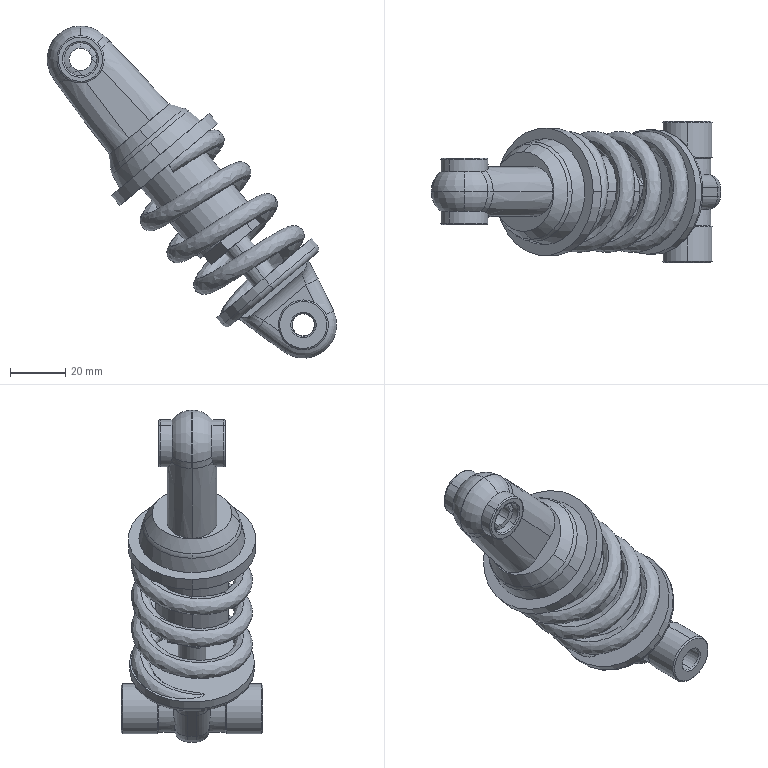Part | SolidWorks | features BaseBody 1 | 1 solid | 143 faces | box 104.348 x 51 x 119.756 mm | volume 93626 mm3 | cylinder 47 | plane 30 | torus 26 | cone 20 | spline 20 | commonest cylinder face diameters 12 x8 17 x8 8 x4 8.2 x4 10 x4 18 x4